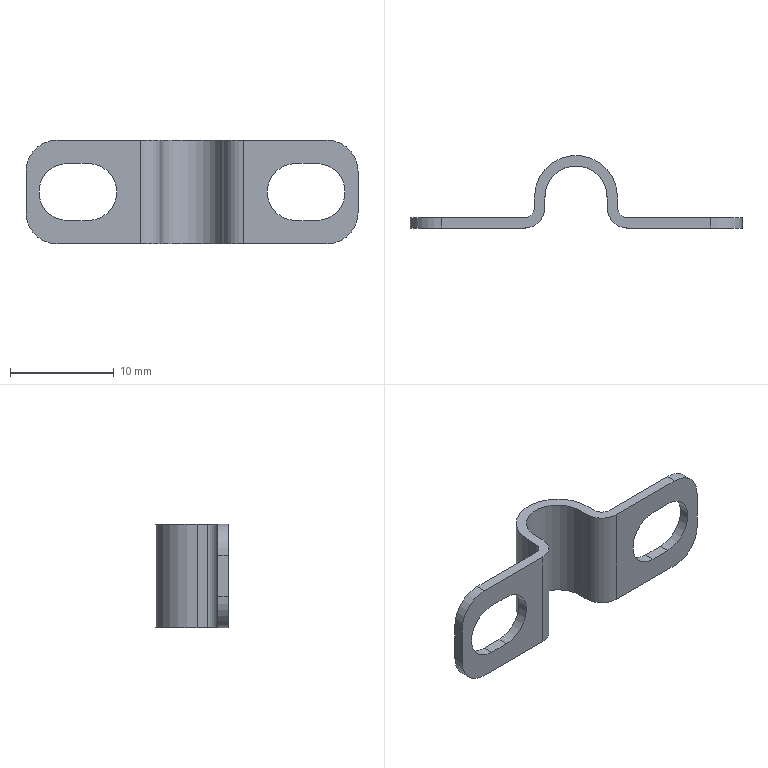Part | NX | features BREP 1 | 1 solid | 30 faces | box 32 x 7 x 10 mm | volume 319.837 mm3 | plane 16 | cylinder 14 | commonest cylinder face diameters 6 x5 5.5 x4 2 x2 4 x2 8 x1
STEP:
#1=CARTESIAN_POINT('',(-12.,0.,-2.75));
#2=VERTEX_POINT('',#1);
#3=CARTESIAN_POINT('',(-12.,0.,2.75));
#4=VERTEX_POINT('',#3);
#5=CARTESIAN_POINT('',(-12.,0.,0.));
#6=DIRECTION('',(0.,1.,0.));
#7=DIRECTION('',(0.,0.,1.));
#8=AXIS2_PLACEMENT_3D('',#5,#6,#7);
#9=CIRCLE('',#8,2.75);
#10=EDGE_CURVE('',#2,#4,#9,.T.);
#11=ORIENTED_EDGE('',*,*,#10,.F.);
#12=CARTESIAN_POINT('',(-12.,1.,-2.75));
#13=VERTEX_POINT('',#12);
#14=CARTESIAN_POINT('',(-12.,-9.,-2.75));
#15=DIRECTION('',(0.,1.,0.));
#16=VECTOR('',#15,1000.);
#17=LINE('',#14,#16);
#18=EDGE_CURVE('',#2,#13,#17,.T.);
#19=ORIENTED_EDGE('',*,*,#18,.T.);
#20=CARTESIAN_POINT('',(-12.,1.,2.75));
#21=VERTEX_POINT('',#20);
#22=CARTESIAN_POINT('',(-12.,1.,0.));
#23=DIRECTION('',(0.,1.,0.));
#24=DIRECTION('',(1.,0.,0.));
#25=AXIS2_PLACEMENT_3D('',#22,#23,#24);
#26=CIRCLE('',#25,2.75);
#27=EDGE_CURVE('',#13,#21,#26,.T.);
#28=ORIENTED_EDGE('',*,*,#27,.T.);
#29=CARTESIAN_POINT('',(-12.,-9.,2.75));
#30=DIRECTION('',(0.,1.,0.));
#31=VECTOR('',#30,1000.);
#32=LINE('',#29,#31);
#33=EDGE_CURVE('',#4,#21,#32,.T.);
#34=ORIENTED_EDGE('',*,*,#33,.F.);
#35=EDGE_LOOP('',(#11,#19,#28,#34));
#36=FACE_BOUND('',#35,.T.);
#37=CARTESIAN_POINT('',(-12.,-9.,0.));
#38=DIRECTION('',(0.,1.,0.));
#39=DIRECTION('',(-1.,0.,0.));
#40=AXIS2_PLACEMENT_3D('',#37,#38,#39);
#41=CYLINDRICAL_SURFACE('',#40,2.75);
#42=ADVANCED_FACE('',(#36),#41,.F.);
#43=CARTESIAN_POINT('',(10.,0.,-2.75));
#44=VERTEX_POINT('',#43);
#45=CARTESIAN_POINT('',(10.,0.,2.75));
#46=VERTEX_POINT('',#45);
#47=CARTESIAN_POINT('',(10.,0.,0.));
#48=DIRECTION('',(0.,1.,0.));
#49=DIRECTION('',(-1.,0.,0.));
#50=AXIS2_PLACEMENT_3D('',#47,#48,#49);
#51=CIRCLE('',#50,2.75);
#52=EDGE_CURVE('',#44,#46,#51,.T.);
#53=ORIENTED_EDGE('',*,*,#52,.F.);
#54=CARTESIAN_POINT('',(10.,1.,-2.75));
#55=VERTEX_POINT('',#54);
#56=CARTESIAN_POINT('',(10.,-9.,-2.75));
#57=DIRECTION('',(0.,1.,0.));
#58=VECTOR('',#57,1000.);
#59=LINE('',#56,#58);
#60=EDGE_CURVE('',#44,#55,#59,.T.);
#61=ORIENTED_EDGE('',*,*,#60,.T.);
#62=CARTESIAN_POINT('',(10.,1.,2.75));
#63=VERTEX_POINT('',#62);
#64=CARTESIAN_POINT('',(10.,1.,0.));
#65=DIRECTION('',(0.,1.,0.));
#66=DIRECTION('',(-1.,0.,0.));
#67=AXIS2_PLACEMENT_3D('',#64,#65,#66);
#68=CIRCLE('',#67,2.75);
#69=EDGE_CURVE('',#55,#63,#68,.T.);
#70=ORIENTED_EDGE('',*,*,#69,.T.);
#71=CARTESIAN_POINT('',(10.,-9.,2.75));
#72=DIRECTION('',(0.,1.,0.));
#73=VECTOR('',#72,1000.);
#74=LINE('',#71,#73);
#75=EDGE_CURVE('',#46,#63,#74,.T.);
#76=ORIENTED_EDGE('',*,*,#75,.F.);
#77=EDGE_LOOP('',(#53,#61,#70,#76));
#78=FACE_BOUND('',#77,.T.);
#79=CARTESIAN_POINT('',(10.,-9.,0.));
#80=DIRECTION('',(0.,1.,0.));
#81=DIRECTION('',(-1.,0.,0.));
#82=AXIS2_PLACEMENT_3D('',#79,#80,#81);
#83=CYLINDRICAL_SURFACE('',#82,2.75);
#84=ADVANCED_FACE('',(#78),#83,.F.);
#85=CARTESIAN_POINT('',(-16.,0.,2.));
#86=VERTEX_POINT('',#85);
#87=CARTESIAN_POINT('',(-16.,0.,-2.));
#88=VERTEX_POINT('',#87);
#89=CARTESIAN_POINT('',(-16.,0.,5.));
#90=DIRECTION('',(0.,0.,-1.));
#91=VECTOR('',#90,1000.);
#92=LINE('',#89,#91);
#93=EDGE_CURVE('',#86,#88,#92,.T.);
#94=ORIENTED_EDGE('',*,*,#93,.F.);
#95=CARTESIAN_POINT('',(-16.,1.,2.));
#96=VERTEX_POINT('',#95);
#97=CARTESIAN_POINT('',(-16.,1.,2.));
#98=DIRECTION('',(0.,1.,0.));
#99=VECTOR('',#98,1000.);
#100=LINE('',#97,#99);
#101=EDGE_CURVE('',#86,#96,#100,.T.);
#102=ORIENTED_EDGE('',*,*,#101,.T.);
#103=CARTESIAN_POINT('',(-16.,1.,-2.));
#104=VERTEX_POINT('',#103);
#105=CARTESIAN_POINT('',(-16.,1.,5.));
#106=DIRECTION('',(0.,0.,-1.));
#107=VECTOR('',#106,1000.);
#108=LINE('',#105,#107);
#109=EDGE_CURVE('',#96,#104,#108,.T.);
#110=ORIENTED_EDGE('',*,*,#109,.T.);
#111=CARTESIAN_POINT('',(-16.,1.,-2.));
#112=DIRECTION('',(0.,-1.,0.));
#113=VECTOR('',#112,1000.);
#114=LINE('',#111,#113);
#115=EDGE_CURVE('',#104,#88,#114,.T.);
#116=ORIENTED_EDGE('',*,*,#115,.T.);
#117=EDGE_LOOP('',(#94,#102,#110,#116));
#118=FACE_BOUND('',#117,.T.);
#119=CARTESIAN_POINT('',(-16.,1.,5.));
#120=DIRECTION('',(1.,0.,0.));
#121=DIRECTION('',(0.,0.,-1.));
#122=AXIS2_PLACEMENT_3D('',#119,#120,#121);
#123=PLANE('',#122);
#124=ADVANCED_FACE('',(#118),#123,.F.);
#125=CARTESIAN_POINT('',(-10.,0.,2.75));
#126=VERTEX_POINT('',#125);
#127=CARTESIAN_POINT('',(-16.,0.,2.75));
#128=DIRECTION('',(1.,0.,0.));
#129=VECTOR('',#128,1000.);
#130=LINE('',#127,#129);
#131=EDGE_CURVE('',#4,#126,#130,.T.);
#132=ORIENTED_EDGE('',*,*,#131,.T.);
#133=CARTESIAN_POINT('',(-10.,0.,-2.75));
#134=VERTEX_POINT('',#133);
#135=CARTESIAN_POINT('',(-10.,0.,0.));
#136=DIRECTION('',(0.,1.,0.));
#137=DIRECTION('',(0.,0.,1.));
#138=AXIS2_PLACEMENT_3D('',#135,#136,#137);
#139=CIRCLE('',#138,2.75);
#140=EDGE_CURVE('',#126,#134,#139,.T.);
#141=ORIENTED_EDGE('',*,*,#140,.T.);
#142=CARTESIAN_POINT('',(-16.,0.,-2.75));
#143=DIRECTION('',(-1.,0.,0.));
#144=VECTOR('',#143,1000.);
#145=LINE('',#142,#144);
#146=EDGE_CURVE('',#134,#2,#145,.T.);
#147=ORIENTED_EDGE('',*,*,#146,.T.);
#148=ORIENTED_EDGE('',*,*,#10,.T.);
#149=EDGE_LOOP('',(#132,#141,#147,#148));
#150=FACE_BOUND('',#149,.T.);
#151=CARTESIAN_POINT('',(-13.,0.,-5.));
#152=VERTEX_POINT('',#151);
#153=CARTESIAN_POINT('',(-5.,0.,-5.));
#154=VERTEX_POINT('',#153);
#155=CARTESIAN_POINT('',(-16.,0.,-5.));
#156=DIRECTION('',(1.,0.,0.));
#157=VECTOR('',#156,1000.);
#158=LINE('',#155,#157);
#159=EDGE_CURVE('',#152,#154,#158,.T.);
#160=ORIENTED_EDGE('',*,*,#159,.T.);
#161=CARTESIAN_POINT('',(-5.,0.,5.));
#162=VERTEX_POINT('',#161);
#163=CARTESIAN_POINT('',(-5.,0.,5.));
#164=DIRECTION('',(0.,0.,1.));
#165=VECTOR('',#164,1000.);
#166=LINE('',#163,#165);
#167=EDGE_CURVE('',#154,#162,#166,.T.);
#168=ORIENTED_EDGE('',*,*,#167,.T.);
#169=CARTESIAN_POINT('',(-13.,0.,5.));
#170=VERTEX_POINT('',#169);
#171=CARTESIAN_POINT('',(-16.,0.,5.));
#172=DIRECTION('',(1.,0.,0.));
#173=VECTOR('',#172,1000.);
#174=LINE('',#171,#173);
#175=EDGE_CURVE('',#170,#162,#174,.T.);
#176=ORIENTED_EDGE('',*,*,#175,.F.);
#177=CARTESIAN_POINT('',(-13.,0.,2.));
#178=DIRECTION('',(0.,-1.,0.));
#179=DIRECTION('',(0.,0.,1.));
#180=AXIS2_PLACEMENT_3D('',#177,#178,#179);
#181=CIRCLE('',#180,3.);
#182=EDGE_CURVE('',#170,#86,#181,.T.);
#183=ORIENTED_EDGE('',*,*,#182,.T.);
#184=ORIENTED_EDGE('',*,*,#93,.T.);
#185=CARTESIAN_POINT('',(-13.,0.,-2.));
#186=DIRECTION('',(0.,-1.,0.));
#187=DIRECTION('',(0.,0.,1.));
#188=AXIS2_PLACEMENT_3D('',#185,#186,#187);
#189=CIRCLE('',#188,3.);
#190=EDGE_CURVE('',#88,#152,#189,.T.);
#191=ORIENTED_EDGE('',*,*,#190,.T.);
#192=EDGE_LOOP('',(#160,#168,#176,#183,#184,#191));
#193=FACE_BOUND('',#192,.T.);
#194=CARTESIAN_POINT('',(-16.,0.,5.));
#195=DIRECTION('',(0.,1.,0.));
#196=DIRECTION('',(0.,0.,1.));
#197=AXIS2_PLACEMENT_3D('',#194,#195,#196);
#198=PLANE('',#197);
#199=ADVANCED_FACE('',(#150,#193),#198,.F.);
#200=CARTESIAN_POINT('',(-3.,2.,5.));
#201=VERTEX_POINT('',#200);
#202=CARTESIAN_POINT('',(-3.,3.,5.));
#203=VERTEX_POINT('',#202);
#204=CARTESIAN_POINT('',(-3.,0.,5.));
#205=DIRECTION('',(0.,1.,0.));
#206=VECTOR('',#205,1000.);
#207=LINE('',#204,#206);
#208=EDGE_CURVE('',#201,#203,#207,.T.);
#209=ORIENTED_EDGE('',*,*,#208,.F.);
#210=CARTESIAN_POINT('',(-3.,2.,-5.));
#211=VERTEX_POINT('',#210);
#212=CARTESIAN_POINT('',(-3.,2.,5.));
#213=DIRECTION('',(0.,0.,-1.));
#214=VECTOR('',#213,1000.);
#215=LINE('',#212,#214);
#216=EDGE_CURVE('',#201,#211,#215,.T.);
#217=ORIENTED_EDGE('',*,*,#216,.T.);
#218=CARTESIAN_POINT('',(-3.,3.,-5.));
#219=VERTEX_POINT('',#218);
#220=CARTESIAN_POINT('',(-3.,0.,-5.));
#221=DIRECTION('',(0.,1.,0.));
#222=VECTOR('',#221,1000.);
#223=LINE('',#220,#222);
#224=EDGE_CURVE('',#211,#219,#223,.T.);
#225=ORIENTED_EDGE('',*,*,#224,.T.);
#226=CARTESIAN_POINT('',(-3.,3.,5.));
#227=DIRECTION('',(0.,0.,-1.));
#228=VECTOR('',#227,1000.);
#229=LINE('',#226,#228);
#230=EDGE_CURVE('',#203,#219,#229,.T.);
#231=ORIENTED_EDGE('',*,*,#230,.F.);
#232=EDGE_LOOP('',(#209,#217,#225,#231));
#233=FACE_BOUND('',#232,.T.);
#234=CARTESIAN_POINT('',(-3.,0.,5.));
#235=DIRECTION('',(-1.,0.,0.));
#236=DIRECTION('',(0.,0.,1.));
#237=AXIS2_PLACEMENT_3D('',#234,#235,#236);
#238=PLANE('',#237);
#239=ADVANCED_FACE('',(#233),#238,.F.);
#240=CARTESIAN_POINT('',(3.,3.,-5.));
#241=VERTEX_POINT('',#240);
#242=CARTESIAN_POINT('',(0.,3.,-5.));
#243=DIRECTION('',(0.,0.,-1.));
#244=DIRECTION('',(1.,0.,0.));
#245=AXIS2_PLACEMENT_3D('',#242,#243,#244);
#246=CIRCLE('',#245,3.);
#247=EDGE_CURVE('',#219,#241,#246,.T.);
#248=ORIENTED_EDGE('',*,*,#247,.T.);
#249=CARTESIAN_POINT('',(3.,3.,5.));
#250=VERTEX_POINT('',#249);
#251=CARTESIAN_POINT('',(3.,3.,5.));
#252=DIRECTION('',(0.,0.,-1.));
#253=VECTOR('',#252,1000.);
#254=LINE('',#251,#253);
#255=EDGE_CURVE('',#250,#241,#254,.T.);
#256=ORIENTED_EDGE('',*,*,#255,.F.);
#257=CARTESIAN_POINT('',(0.,3.,5.));
#258=DIRECTION('',(0.,0.,-1.));
#259=DIRECTION('',(1.,0.,0.));
#260=AXIS2_PLACEMENT_3D('',#257,#258,#259);
#261=CIRCLE('',#260,3.);
#262=EDGE_CURVE('',#203,#250,#261,.T.);
#263=ORIENTED_EDGE('',*,*,#262,.F.);
#264=ORIENTED_EDGE('',*,*,#230,.T.);
#265=EDGE_LOOP('',(#248,#256,#263,#264));
#266=FACE_BOUND('',#265,.T.);
#267=CARTESIAN_POINT('',(0.,3.,5.));
#268=DIRECTION('',(0.,0.,-1.));
#269=DIRECTION('',(-1.,0.,0.));
#270=AXIS2_PLACEMENT_3D('',#267,#268,#269);
#271=CYLINDRICAL_SURFACE('',#270,3.);
#272=ADVANCED_FACE('',(#266),#271,.F.);
#273=CARTESIAN_POINT('',(3.,2.,-5.));
#274=VERTEX_POINT('',#273);
#275=CARTESIAN_POINT('',(3.,0.,-5.));
#276=DIRECTION('',(0.,-1.,0.));
#277=VECTOR('',#276,1000.);
#278=LINE('',#275,#277);
#279=EDGE_CURVE('',#241,#274,#278,.T.);
#280=ORIENTED_EDGE('',*,*,#279,.T.);
#281=CARTESIAN_POINT('',(3.,2.,5.));
#282=VERTEX_POINT('',#281);
#283=CARTESIAN_POINT('',(3.,2.,5.));
#284=DIRECTION('',(0.,0.,1.));
#285=VECTOR('',#284,1000.);
#286=LINE('',#283,#285);
#287=EDGE_CURVE('',#274,#282,#286,.T.);
#288=ORIENTED_EDGE('',*,*,#287,.T.);
#289=CARTESIAN_POINT('',(3.,0.,5.));
#290=DIRECTION('',(0.,-1.,0.));
#291=VECTOR('',#290,1000.);
#292=LINE('',#289,#291);
#293=EDGE_CURVE('',#250,#282,#292,.T.);
#294=ORIENTED_EDGE('',*,*,#293,.F.);
#295=ORIENTED_EDGE('',*,*,#255,.T.);
#296=EDGE_LOOP('',(#280,#288,#294,#295));
#297=FACE_BOUND('',#296,.T.);
#298=CARTESIAN_POINT('',(3.,0.,5.));
#299=DIRECTION('',(1.,0.,0.));
#300=DIRECTION('',(0.,1.,0.));
#301=AXIS2_PLACEMENT_3D('',#298,#299,#300);
#302=PLANE('',#301);
#303=ADVANCED_FACE('',(#297),#302,.F.);
#304=CARTESIAN_POINT('',(12.,0.,-2.75));
#305=VERTEX_POINT('',#304);
#306=CARTESIAN_POINT('',(3.,0.,-2.75));
#307=DIRECTION('',(-1.,0.,0.));
#308=VECTOR('',#307,1000.);
#309=LINE('',#306,#308);
#310=EDGE_CURVE('',#305,#44,#309,.T.);
#311=ORIENTED_EDGE('',*,*,#310,.T.);
#312=ORIENTED_EDGE('',*,*,#52,.T.);
#313=CARTESIAN_POINT('',(12.,0.,2.75));
#314=VERTEX_POINT('',#313);
#315=CARTESIAN_POINT('',(3.,0.,2.75));
#316=DIRECTION('',(1.,0.,0.));
#317=VECTOR('',#316,1000.);
#318=LINE('',#315,#317);
#319=EDGE_CURVE('',#46,#314,#318,.T.);
#320=ORIENTED_EDGE('',*,*,#319,.T.);
#321=CARTESIAN_POINT('',(12.,0.,0.));
#322=DIRECTION('',(0.,1.,0.));
#323=DIRECTION('',(-1.,0.,0.));
#324=AXIS2_PLACEMENT_3D('',#321,#322,#323);
#325=CIRCLE('',#324,2.75);
#326=EDGE_CURVE('',#314,#305,#325,.T.);
#327=ORIENTED_EDGE('',*,*,#326,.T.);
#328=EDGE_LOOP('',(#311,#312,#320,#327));
#329=FACE_BOUND('',#328,.T.);
#330=CARTESIAN_POINT('',(5.,0.,5.));
#331=VERTEX_POINT('',#330);
#332=CARTESIAN_POINT('',(13.,0.,5.));
#333=VERTEX_POINT('',#332);
#334=CARTESIAN_POINT('',(3.,0.,5.));
#335=DIRECTION('',(1.,0.,0.));
#336=VECTOR('',#335,1000.);
#337=LINE('',#334,#336);
#338=EDGE_CURVE('',#331,#333,#337,.T.);
#339=ORIENTED_EDGE('',*,*,#338,.F.);
#340=CARTESIAN_POINT('',(5.,0.,-5.));
#341=VERTEX_POINT('',#340);
#342=CARTESIAN_POINT('',(5.,0.,5.));
#343=DIRECTION('',(0.,0.,-1.));
#344=VECTOR('',#343,1000.);
#345=LINE('',#342,#344);
#346=EDGE_CURVE('',#331,#341,#345,.T.);
#347=ORIENTED_EDGE('',*,*,#346,.T.);
#348=CARTESIAN_POINT('',(13.,0.,-5.));
#349=VERTEX_POINT('',#348);
#350=CARTESIAN_POINT('',(3.,0.,-5.));
#351=DIRECTION('',(1.,0.,0.));
#352=VECTOR('',#351,1000.);
#353=LINE('',#350,#352);
#354=EDGE_CURVE('',#341,#349,#353,.T.);
#355=ORIENTED_EDGE('',*,*,#354,.T.);
#356=CARTESIAN_POINT('',(16.,0.,-2.));
#357=VERTEX_POINT('',#356);
#358=CARTESIAN_POINT('',(13.,0.,-2.));
#359=DIRECTION('',(0.,-1.,0.));
#360=DIRECTION('',(-1.,0.,0.));
#361=AXIS2_PLACEMENT_3D('',#358,#359,#360);
#362=CIRCLE('',#361,3.);
#363=EDGE_CURVE('',#349,#357,#362,.T.);
#364=ORIENTED_EDGE('',*,*,#363,.T.);
#365=CARTESIAN_POINT('',(16.,0.,2.));
#366=VERTEX_POINT('',#365);
#367=CARTESIAN_POINT('',(16.,0.,5.));
#368=DIRECTION('',(0.,0.,-1.));
#369=VECTOR('',#368,1000.);
#370=LINE('',#367,#369);
#371=EDGE_CURVE('',#366,#357,#370,.T.);
#372=ORIENTED_EDGE('',*,*,#371,.F.);
#373=CARTESIAN_POINT('',(13.,0.,2.));
#374=DIRECTION('',(0.,-1.,0.));
#375=DIRECTION('',(-1.,0.,0.));
#376=AXIS2_PLACEMENT_3D('',#373,#374,#375);
#377=CIRCLE('',#376,3.);
#378=EDGE_CURVE('',#366,#333,#377,.T.);
#379=ORIENTED_EDGE('',*,*,#378,.T.);
#380=EDGE_LOOP('',(#339,#347,#355,#364,#372,#379));
#381=FACE_BOUND('',#380,.T.);
#382=CARTESIAN_POINT('',(3.,0.,5.));
#383=DIRECTION('',(0.,1.,0.));
#384=DIRECTION('',(-1.,0.,0.));
#385=AXIS2_PLACEMENT_3D('',#382,#383,#384);
#386=PLANE('',#385);
#387=ADVANCED_FACE('',(#329,#381),#386,.F.);
#388=ORIENTED_EDGE('',*,*,#371,.T.);
#389=CARTESIAN_POINT('',(16.,1.,-2.));
#390=VERTEX_POINT('',#389);
#391=CARTESIAN_POINT('',(16.,0.,-2.));
#392=DIRECTION('',(0.,1.,0.));
#393=VECTOR('',#392,1000.);
#394=LINE('',#391,#393);
#395=EDGE_CURVE('',#357,#390,#394,.T.);
#396=ORIENTED_EDGE('',*,*,#395,.T.);
#397=CARTESIAN_POINT('',(16.,1.,2.));
#398=VERTEX_POINT('',#397);
#399=CARTESIAN_POINT('',(16.,1.,5.));
#400=DIRECTION('',(0.,0.,-1.));
#401=VECTOR('',#400,1000.);
#402=LINE('',#399,#401);
#403=EDGE_CURVE('',#398,#390,#402,.T.);
#404=ORIENTED_EDGE('',*,*,#403,.F.);
#405=CARTESIAN_POINT('',(16.,0.,2.));
#406=DIRECTION('',(0.,-1.,0.));
#407=VECTOR('',#406,1000.);
#408=LINE('',#405,#407);
#409=EDGE_CURVE('',#398,#366,#408,.T.);
#410=ORIENTED_EDGE('',*,*,#409,.T.);
#411=EDGE_LOOP('',(#388,#396,#404,#410));
#412=FACE_BOUND('',#411,.T.);
#413=CARTESIAN_POINT('',(16.,0.,5.));
#414=DIRECTION('',(-1.,0.,0.));
#415=DIRECTION('',(0.,0.,1.));
#416=AXIS2_PLACEMENT_3D('',#413,#414,#415);
#417=PLANE('',#416);
#418=ADVANCED_FACE('',(#412),#417,.F.);
#419=CARTESIAN_POINT('',(12.,1.,2.75));
#420=VERTEX_POINT('',#419);
#421=CARTESIAN_POINT('',(10.,1.,2.75));
#422=DIRECTION('',(1.,0.,0.));
#423=VECTOR('',#422,1000.);
#424=LINE('',#421,#423);
#425=EDGE_CURVE('',#63,#420,#424,.T.);
#426=ORIENTED_EDGE('',*,*,#425,.F.);
#427=ORIENTED_EDGE('',*,*,#69,.F.);
#428=CARTESIAN_POINT('',(12.,1.,-2.75));
#429=VERTEX_POINT('',#428);
#430=CARTESIAN_POINT('',(10.,1.,-2.75));
#431=DIRECTION('',(-1.,0.,0.));
#432=VECTOR('',#431,1000.);
#433=LINE('',#430,#432);
#434=EDGE_CURVE('',#429,#55,#433,.T.);
#435=ORIENTED_EDGE('',*,*,#434,.F.);
#436=CARTESIAN_POINT('',(12.,1.,0.));
#437=DIRECTION('',(0.,1.,0.));
#438=DIRECTION('',(-1.,0.,0.));
#439=AXIS2_PLACEMENT_3D('',#436,#437,#438);
#440=CIRCLE('',#439,2.75);
#441=EDGE_CURVE('',#420,#429,#440,.T.);
#442=ORIENTED_EDGE('',*,*,#441,.F.);
#443=EDGE_LOOP('',(#426,#427,#435,#442));
#444=FACE_BOUND('',#443,.T.);
#445=CARTESIAN_POINT('',(13.,1.,-5.));
#446=VERTEX_POINT('',#445);
#447=CARTESIAN_POINT('',(5.,1.,-5.));
#448=VERTEX_POINT('',#447);
#449=CARTESIAN_POINT('',(4.,1.,-5.));
#450=DIRECTION('',(-1.,0.,0.));
#451=VECTOR('',#450,1000.);
#452=LINE('',#449,#451);
#453=EDGE_CURVE('',#446,#448,#452,.T.);
#454=ORIENTED_EDGE('',*,*,#453,.T.);
#455=CARTESIAN_POINT('',(5.,1.,5.));
#456=VERTEX_POINT('',#455);
#457=CARTESIAN_POINT('',(5.,1.,5.));
#458=DIRECTION('',(0.,0.,1.));
#459=VECTOR('',#458,1000.);
#460=LINE('',#457,#459);
#461=EDGE_CURVE('',#448,#456,#460,.T.);
#462=ORIENTED_EDGE('',*,*,#461,.T.);
#463=CARTESIAN_POINT('',(13.,1.,5.));
#464=VERTEX_POINT('',#463);
#465=CARTESIAN_POINT('',(4.,1.,5.));
#466=DIRECTION('',(-1.,0.,0.));
#467=VECTOR('',#466,1000.);
#468=LINE('',#465,#467);
#469=EDGE_CURVE('',#464,#456,#468,.T.);
#470=ORIENTED_EDGE('',*,*,#469,.F.);
#471=CARTESIAN_POINT('',(13.,1.,2.));
#472=DIRECTION('',(0.,1.,0.));
#473=DIRECTION('',(1.,0.,0.));
#474=AXIS2_PLACEMENT_3D('',#471,#472,#473);
#475=CIRCLE('',#474,3.);
#476=EDGE_CURVE('',#464,#398,#475,.T.);
#477=ORIENTED_EDGE('',*,*,#476,.T.);
#478=ORIENTED_EDGE('',*,*,#403,.T.);
#479=CARTESIAN_POINT('',(13.,1.,-2.));
#480=DIRECTION('',(0.,1.,0.));
#481=DIRECTION('',(1.,0.,0.));
#482=AXIS2_PLACEMENT_3D('',#479,#480,#481);
#483=CIRCLE('',#482,3.);
#484=EDGE_CURVE('',#390,#446,#483,.T.);
#485=ORIENTED_EDGE('',*,*,#484,.T.);
#486=EDGE_LOOP('',(#454,#462,#470,#477,#478,#485));
#487=FACE_BOUND('',#486,.T.);
#488=CARTESIAN_POINT('',(4.,1.,5.));
#489=DIRECTION('',(0.,-1.,0.));
#490=DIRECTION('',(1.,0.,0.));
#491=AXIS2_PLACEMENT_3D('',#488,#489,#490);
#492=PLANE('',#491);
#493=ADVANCED_FACE('',(#444,#487),#492,.F.);
#494=CARTESIAN_POINT('',(4.,2.,5.));
#495=VERTEX_POINT('',#494);
#496=CARTESIAN_POINT('',(4.,3.,5.));
#497=VERTEX_POINT('',#496);
#498=CARTESIAN_POINT('',(4.,1.,5.));
#499=DIRECTION('',(0.,1.,0.));
#500=VECTOR('',#499,1000.);
#501=LINE('',#498,#500);
#502=EDGE_CURVE('',#495,#497,#501,.T.);
#503=ORIENTED_EDGE('',*,*,#502,.F.);
#504=CARTESIAN_POINT('',(4.,2.,-5.));
#505=VERTEX_POINT('',#504);
#506=CARTESIAN_POINT('',(4.,2.,-5.));
#507=DIRECTION('',(0.,0.,-1.));
#508=VECTOR('',#507,1000.);
#509=LINE('',#506,#508);
#510=EDGE_CURVE('',#495,#505,#509,.T.);
#511=ORIENTED_EDGE('',*,*,#510,.T.);
#512=CARTESIAN_POINT('',(4.,3.,-5.));
#513=VERTEX_POINT('',#512);
#514=CARTESIAN_POINT('',(4.,1.,-5.));
#515=DIRECTION('',(0.,1.,0.));
#516=VECTOR('',#515,1000.);
#517=LINE('',#514,#516);
#518=EDGE_CURVE('',#505,#513,#517,.T.);
#519=ORIENTED_EDGE('',*,*,#518,.T.);
#520=CARTESIAN_POINT('',(4.,3.,5.));
#521=DIRECTION('',(0.,0.,-1.));
#522=VECTOR('',#521,1000.);
#523=LINE('',#520,#522);
#524=EDGE_CURVE('',#497,#513,#523,.T.);
#525=ORIENTED_EDGE('',*,*,#524,.F.);
#526=EDGE_LOOP('',(#503,#511,#519,#525));
#527=FACE_BOUND('',#526,.T.);
#528=CARTESIAN_POINT('',(4.,1.,5.));
#529=DIRECTION('',(-1.,0.,0.));
#530=DIRECTION('',(0.,0.,1.));
#531=AXIS2_PLACEMENT_3D('',#528,#529,#530);
#532=PLANE('',#531);
#533=ADVANCED_FACE('',(#527),#532,.F.);
#534=CARTESIAN_POINT('',(-4.,3.,-5.));
#535=VERTEX_POINT('',#534);
#536=CARTESIAN_POINT('',(0.,3.,-5.));
#537=DIRECTION('',(0.,0.,1.));
#538=DIRECTION('',(1.,0.,0.));
#539=AXIS2_PLACEMENT_3D('',#536,#537,#538);
#540=CIRCLE('',#539,4.);
#541=EDGE_CURVE('',#513,#535,#540,.T.);
#542=ORIENTED_EDGE('',*,*,#541,.T.);
#543=CARTESIAN_POINT('',(-4.,3.,5.));
#544=VERTEX_POINT('',#543);
#545=CARTESIAN_POINT('',(-4.,3.,5.));
#546=DIRECTION('',(0.,0.,-1.));
#547=VECTOR('',#546,1000.);
#548=LINE('',#545,#547);
#549=EDGE_CURVE('',#544,#535,#548,.T.);
#550=ORIENTED_EDGE('',*,*,#549,.F.);
#551=CARTESIAN_POINT('',(0.,3.,5.));
#552=DIRECTION('',(0.,0.,1.));
#553=DIRECTION('',(1.,0.,0.));
#554=AXIS2_PLACEMENT_3D('',#551,#552,#553);
#555=CIRCLE('',#554,4.);
#556=EDGE_CURVE('',#497,#544,#555,.T.);
#557=ORIENTED_EDGE('',*,*,#556,.F.);
#558=ORIENTED_EDGE('',*,*,#524,.T.);
#559=EDGE_LOOP('',(#542,#550,#557,#558));
#560=FACE_BOUND('',#559,.T.);
#561=CARTESIAN_POINT('',(0.,3.,5.));
#562=DIRECTION('',(0.,0.,-1.));
#563=DIRECTION('',(-1.,0.,0.));
#564=AXIS2_PLACEMENT_3D('',#561,#562,#563);
#565=CYLINDRICAL_SURFACE('',#564,4.);
#566=ADVANCED_FACE('',(#560),#565,.T.);
#567=CARTESIAN_POINT('',(-4.,2.,-5.));
#568=VERTEX_POINT('',#567);
#569=CARTESIAN_POINT('',(-4.,1.,-5.));
#570=DIRECTION('',(0.,-1.,0.));
#571=VECTOR('',#570,1000.);
#572=LINE('',#569,#571);
#573=EDGE_CURVE('',#535,#568,#572,.T.);
#574=ORIENTED_EDGE('',*,*,#573,.T.);
#575=CARTESIAN_POINT('',(-4.,2.,5.));
#576=VERTEX_POINT('',#575);
#577=CARTESIAN_POINT('',(-4.,2.,5.));
#578=DIRECTION('',(0.,0.,1.));
#579=VECTOR('',#578,1000.);
#580=LINE('',#577,#579);
#581=EDGE_CURVE('',#568,#576,#580,.T.);
#582=ORIENTED_EDGE('',*,*,#581,.T.);
#583=CARTESIAN_POINT('',(-4.,1.,5.));
#584=DIRECTION('',(0.,-1.,0.));
#585=VECTOR('',#584,1000.);
#586=LINE('',#583,#585);
#587=EDGE_CURVE('',#544,#576,#586,.T.);
#588=ORIENTED_EDGE('',*,*,#587,.F.);
#589=ORIENTED_EDGE('',*,*,#549,.T.);
#590=EDGE_LOOP('',(#574,#582,#588,#589));
#591=FACE_BOUND('',#590,.T.);
#592=CARTESIAN_POINT('',(-4.,1.,5.));
#593=DIRECTION('',(1.,0.,0.));
#594=DIRECTION('',(0.,1.,0.));
#595=AXIS2_PLACEMENT_3D('',#592,#593,#594);
#596=PLANE('',#595);
#597=ADVANCED_FACE('',(#591),#596,.F.);
#598=CARTESIAN_POINT('',(-10.,1.,-2.75));
#599=VERTEX_POINT('',#598);
#600=CARTESIAN_POINT('',(-10.,1.,-2.75));
#601=DIRECTION('',(-1.,0.,0.));
#602=VECTOR('',#601,1000.);
#603=LINE('',#600,#602);
#604=EDGE_CURVE('',#599,#13,#603,.T.);
#605=ORIENTED_EDGE('',*,*,#604,.F.);
#606=CARTESIAN_POINT('',(-10.,1.,2.75));
#607=VERTEX_POINT('',#606);
#608=CARTESIAN_POINT('',(-10.,1.,0.));
#609=DIRECTION('',(0.,1.,0.));
#610=DIRECTION('',(1.,0.,0.));
#611=AXIS2_PLACEMENT_3D('',#608,#609,#610);
#612=CIRCLE('',#611,2.75);
#613=EDGE_CURVE('',#607,#599,#612,.T.);
#614=ORIENTED_EDGE('',*,*,#613,.F.);
#615=CARTESIAN_POINT('',(-10.,1.,2.75));
#616=DIRECTION('',(1.,0.,0.));
#617=VECTOR('',#616,1000.);
#618=LINE('',#615,#617);
#619=EDGE_CURVE('',#21,#607,#618,.T.);
#620=ORIENTED_EDGE('',*,*,#619,.F.);
#621=ORIENTED_EDGE('',*,*,#27,.F.);
#622=EDGE_LOOP('',(#605,#614,#620,#621));
#623=FACE_BOUND('',#622,.T.);
#624=CARTESIAN_POINT('',(-5.,1.,5.));
#625=VERTEX_POINT('',#624);
#626=CARTESIAN_POINT('',(-13.,1.,5.));
#627=VERTEX_POINT('',#626);
#628=CARTESIAN_POINT('',(-16.,1.,5.));
#629=DIRECTION('',(-1.,0.,0.));
#630=VECTOR('',#629,1000.);
#631=LINE('',#628,#630);
#632=EDGE_CURVE('',#625,#627,#631,.T.);
#633=ORIENTED_EDGE('',*,*,#632,.F.);
#634=CARTESIAN_POINT('',(-5.,1.,-5.));
#635=VERTEX_POINT('',#634);
#636=CARTESIAN_POINT('',(-5.,1.,-5.));
#637=DIRECTION('',(0.,0.,-1.));
#638=VECTOR('',#637,1000.);
#639=LINE('',#636,#638);
#640=EDGE_CURVE('',#625,#635,#639,.T.);
#641=ORIENTED_EDGE('',*,*,#640,.T.);
#642=CARTESIAN_POINT('',(-13.,1.,-5.));
#643=VERTEX_POINT('',#642);
#644=CARTESIAN_POINT('',(-16.,1.,-5.));
#645=DIRECTION('',(-1.,0.,0.));
#646=VECTOR('',#645,1000.);
#647=LINE('',#644,#646);
#648=EDGE_CURVE('',#635,#643,#647,.T.);
#649=ORIENTED_EDGE('',*,*,#648,.T.);
#650=CARTESIAN_POINT('',(-13.,1.,-2.));
#651=DIRECTION('',(0.,1.,0.));
#652=DIRECTION('',(0.,0.,-1.));
#653=AXIS2_PLACEMENT_3D('',#650,#651,#652);
#654=CIRCLE('',#653,3.);
#655=EDGE_CURVE('',#643,#104,#654,.T.);
#656=ORIENTED_EDGE('',*,*,#655,.T.);
#657=ORIENTED_EDGE('',*,*,#109,.F.);
#658=CARTESIAN_POINT('',(-13.,1.,2.));
#659=DIRECTION('',(0.,1.,0.));
#660=DIRECTION('',(0.,0.,-1.));
#661=AXIS2_PLACEMENT_3D('',#658,#659,#660);
#662=CIRCLE('',#661,3.);
#663=EDGE_CURVE('',#96,#627,#662,.T.);
#664=ORIENTED_EDGE('',*,*,#663,.T.);
#665=EDGE_LOOP('',(#633,#641,#649,#656,#657,#664));
#666=FACE_BOUND('',#665,.T.);
#667=CARTESIAN_POINT('',(-16.,1.,5.));
#668=DIRECTION('',(0.,-1.,0.));
#669=DIRECTION('',(0.,0.,-1.));
#670=AXIS2_PLACEMENT_3D('',#667,#668,#669);
#671=PLANE('',#670);
#672=ADVANCED_FACE('',(#623,#666),#671,.F.);
#673=ORIENTED_EDGE('',*,*,#175,.T.);
#674=CARTESIAN_POINT('',(-5.,2.,5.));
#675=DIRECTION('',(0.,0.,1.));
#676=DIRECTION('',(1.,0.,0.));
#677=AXIS2_PLACEMENT_3D('',#674,#675,#676);
#678=CIRCLE('',#677,2.);
#679=EDGE_CURVE('',#162,#201,#678,.T.);
#680=ORIENTED_EDGE('',*,*,#679,.T.);
#681=ORIENTED_EDGE('',*,*,#208,.T.);
#682=ORIENTED_EDGE('',*,*,#262,.T.);
#683=ORIENTED_EDGE('',*,*,#293,.T.);
#684=CARTESIAN_POINT('',(5.,2.,5.));
#685=DIRECTION('',(0.,0.,1.));
#686=DIRECTION('',(1.,0.,0.));
#687=AXIS2_PLACEMENT_3D('',#684,#685,#686);
#688=CIRCLE('',#687,2.);
#689=EDGE_CURVE('',#282,#331,#688,.T.);
#690=ORIENTED_EDGE('',*,*,#689,.T.);
#691=ORIENTED_EDGE('',*,*,#338,.T.);
#692=CARTESIAN_POINT('',(13.,1.,5.));
#693=DIRECTION('',(0.,1.,0.));
#694=VECTOR('',#693,1000.);
#695=LINE('',#692,#694);
#696=EDGE_CURVE('',#333,#464,#695,.T.);
#697=ORIENTED_EDGE('',*,*,#696,.T.);
#698=ORIENTED_EDGE('',*,*,#469,.T.);
#699=CARTESIAN_POINT('',(5.,2.,5.));
#700=DIRECTION('',(0.,0.,-1.));
#701=DIRECTION('',(1.,0.,0.));
#702=AXIS2_PLACEMENT_3D('',#699,#700,#701);
#703=CIRCLE('',#702,1.);
#704=EDGE_CURVE('',#456,#495,#703,.T.);
#705=ORIENTED_EDGE('',*,*,#704,.T.);
#706=ORIENTED_EDGE('',*,*,#502,.T.);
#707=ORIENTED_EDGE('',*,*,#556,.T.);
#708=ORIENTED_EDGE('',*,*,#587,.T.);
#709=CARTESIAN_POINT('',(-5.,2.,5.));
#710=DIRECTION('',(0.,0.,-1.));
#711=DIRECTION('',(1.,0.,0.));
#712=AXIS2_PLACEMENT_3D('',#709,#710,#711);
#713=CIRCLE('',#712,1.);
#714=EDGE_CURVE('',#576,#625,#713,.T.);
#715=ORIENTED_EDGE('',*,*,#714,.T.);
#716=ORIENTED_EDGE('',*,*,#632,.T.);
#717=CARTESIAN_POINT('',(-13.,0.,5.));
#718=DIRECTION('',(0.,-1.,0.));
#719=VECTOR('',#718,1000.);
#720=LINE('',#717,#719);
#721=EDGE_CURVE('',#627,#170,#720,.T.);
#722=ORIENTED_EDGE('',*,*,#721,.T.);
#723=EDGE_LOOP('',(#673,#680,#681,#682,#683,#690,#691,#697,#698,#705,#706,#707,#708,#715,#716,#722));
#724=FACE_BOUND('',#723,.T.);
#725=CARTESIAN_POINT('',(0.,3.,5.));
#726=DIRECTION('',(0.,0.,1.));
#727=DIRECTION('',(1.,0.,0.));
#728=AXIS2_PLACEMENT_3D('',#725,#726,#727);
#729=PLANE('',#728);
#730=ADVANCED_FACE('',(#724),#729,.T.);
#731=ORIENTED_EDGE('',*,*,#224,.F.);
#732=CARTESIAN_POINT('',(-5.,2.,-5.));
#733=DIRECTION('',(0.,0.,-1.));
#734=DIRECTION('',(1.,0.,0.));
#735=AXIS2_PLACEMENT_3D('',#732,#733,#734);
#736=CIRCLE('',#735,2.);
#737=EDGE_CURVE('',#211,#154,#736,.T.);
#738=ORIENTED_EDGE('',*,*,#737,.T.);
#739=ORIENTED_EDGE('',*,*,#159,.F.);
#740=CARTESIAN_POINT('',(-13.,3.,-5.));
#741=DIRECTION('',(0.,1.,0.));
#742=VECTOR('',#741,1000.);
#743=LINE('',#740,#742);
#744=EDGE_CURVE('',#152,#643,#743,.T.);
#745=ORIENTED_EDGE('',*,*,#744,.T.);
#746=ORIENTED_EDGE('',*,*,#648,.F.);
#747=CARTESIAN_POINT('',(-5.,2.,-5.));
#748=DIRECTION('',(0.,0.,1.));
#749=DIRECTION('',(1.,0.,0.));
#750=AXIS2_PLACEMENT_3D('',#747,#748,#749);
#751=CIRCLE('',#750,1.);
#752=EDGE_CURVE('',#635,#568,#751,.T.);
#753=ORIENTED_EDGE('',*,*,#752,.T.);
#754=ORIENTED_EDGE('',*,*,#573,.F.);
#755=ORIENTED_EDGE('',*,*,#541,.F.);
#756=ORIENTED_EDGE('',*,*,#518,.F.);
#757=CARTESIAN_POINT('',(5.,2.,-5.));
#758=DIRECTION('',(0.,0.,1.));
#759=DIRECTION('',(1.,0.,0.));
#760=AXIS2_PLACEMENT_3D('',#757,#758,#759);
#761=CIRCLE('',#760,1.);
#762=EDGE_CURVE('',#505,#448,#761,.T.);
#763=ORIENTED_EDGE('',*,*,#762,.T.);
#764=ORIENTED_EDGE('',*,*,#453,.F.);
#765=CARTESIAN_POINT('',(13.,3.,-5.));
#766=DIRECTION('',(0.,-1.,0.));
#767=VECTOR('',#766,1000.);
#768=LINE('',#765,#767);
#769=EDGE_CURVE('',#446,#349,#768,.T.);
#770=ORIENTED_EDGE('',*,*,#769,.T.);
#771=ORIENTED_EDGE('',*,*,#354,.F.);
#772=CARTESIAN_POINT('',(5.,2.,-5.));
#773=DIRECTION('',(0.,0.,-1.));
#774=DIRECTION('',(1.,0.,0.));
#775=AXIS2_PLACEMENT_3D('',#772,#773,#774);
#776=CIRCLE('',#775,2.);
#777=EDGE_CURVE('',#341,#274,#776,.T.);
#778=ORIENTED_EDGE('',*,*,#777,.T.);
#779=ORIENTED_EDGE('',*,*,#279,.F.);
#780=ORIENTED_EDGE('',*,*,#247,.F.);
#781=EDGE_LOOP('',(#731,#738,#739,#745,#746,#753,#754,#755,#756,#763,#764,#770,#771,#778,#779,#780));
#782=FACE_BOUND('',#781,.T.);
#783=CARTESIAN_POINT('',(0.,3.,-5.));
#784=DIRECTION('',(0.,0.,1.));
#785=DIRECTION('',(1.,0.,0.));
#786=AXIS2_PLACEMENT_3D('',#783,#784,#785);
#787=PLANE('',#786);
#788=ADVANCED_FACE('',(#782),#787,.F.);
#789=CARTESIAN_POINT('',(12.,-9.,2.75));
#790=DIRECTION('',(0.,1.,0.));
#791=VECTOR('',#790,1000.);
#792=LINE('',#789,#791);
#793=EDGE_CURVE('',#314,#420,#792,.T.);
#794=ORIENTED_EDGE('',*,*,#793,.T.);
#795=ORIENTED_EDGE('',*,*,#441,.T.);
#796=CARTESIAN_POINT('',(12.,-9.,-2.75));
#797=DIRECTION('',(0.,1.,0.));
#798=VECTOR('',#797,1000.);
#799=LINE('',#796,#798);
#800=EDGE_CURVE('',#305,#429,#799,.T.);
#801=ORIENTED_EDGE('',*,*,#800,.F.);
#802=ORIENTED_EDGE('',*,*,#326,.F.);
#803=EDGE_LOOP('',(#794,#795,#801,#802));
#804=FACE_BOUND('',#803,.T.);
#805=CARTESIAN_POINT('',(12.,-9.,0.));
#806=DIRECTION('',(0.,1.,0.));
#807=DIRECTION('',(-1.,0.,0.));
#808=AXIS2_PLACEMENT_3D('',#805,#806,#807);
#809=CYLINDRICAL_SURFACE('',#808,2.75);
#810=ADVANCED_FACE('',(#804),#809,.F.);
#811=ORIENTED_EDGE('',*,*,#800,.T.);
#812=ORIENTED_EDGE('',*,*,#434,.T.);
#813=ORIENTED_EDGE('',*,*,#60,.F.);
#814=ORIENTED_EDGE('',*,*,#310,.F.);
#815=EDGE_LOOP('',(#811,#812,#813,#814));
#816=FACE_BOUND('',#815,.T.);
#817=CARTESIAN_POINT('',(10.,-9.,-2.75));
#818=DIRECTION('',(0.,0.,-1.));
#819=DIRECTION('',(-1.,0.,0.));
#820=AXIS2_PLACEMENT_3D('',#817,#818,#819);
#821=PLANE('',#820);
#822=ADVANCED_FACE('',(#816),#821,.F.);
#823=ORIENTED_EDGE('',*,*,#75,.T.);
#824=ORIENTED_EDGE('',*,*,#425,.T.);
#825=ORIENTED_EDGE('',*,*,#793,.F.);
#826=ORIENTED_EDGE('',*,*,#319,.F.);
#827=EDGE_LOOP('',(#823,#824,#825,#826));
#828=FACE_BOUND('',#827,.T.);
#829=CARTESIAN_POINT('',(10.,-9.,2.75));
#830=DIRECTION('',(0.,0.,1.));
#831=DIRECTION('',(1.,0.,0.));
#832=AXIS2_PLACEMENT_3D('',#829,#830,#831);
#833=PLANE('',#832);
#834=ADVANCED_FACE('',(#828),#833,.F.);
#835=CARTESIAN_POINT('',(-10.,-9.,2.75));
#836=DIRECTION('',(0.,1.,0.));
#837=VECTOR('',#836,1000.);
#838=LINE('',#835,#837);
#839=EDGE_CURVE('',#126,#607,#838,.T.);
#840=ORIENTED_EDGE('',*,*,#839,.T.);
#841=ORIENTED_EDGE('',*,*,#613,.T.);
#842=CARTESIAN_POINT('',(-10.,-9.,-2.75));
#843=DIRECTION('',(0.,1.,0.));
#844=VECTOR('',#843,1000.);
#845=LINE('',#842,#844);
#846=EDGE_CURVE('',#134,#599,#845,.T.);
#847=ORIENTED_EDGE('',*,*,#846,.F.);
#848=ORIENTED_EDGE('',*,*,#140,.F.);
#849=EDGE_LOOP('',(#840,#841,#847,#848));
#850=FACE_BOUND('',#849,.T.);
#851=CARTESIAN_POINT('',(-10.,-9.,0.));
#852=DIRECTION('',(0.,1.,0.));
#853=DIRECTION('',(-1.,0.,0.));
#854=AXIS2_PLACEMENT_3D('',#851,#852,#853);
#855=CYLINDRICAL_SURFACE('',#854,2.75);
#856=ADVANCED_FACE('',(#850),#855,.F.);
#857=ORIENTED_EDGE('',*,*,#33,.T.);
#858=ORIENTED_EDGE('',*,*,#619,.T.);
#859=ORIENTED_EDGE('',*,*,#839,.F.);
#860=ORIENTED_EDGE('',*,*,#131,.F.);
#861=EDGE_LOOP('',(#857,#858,#859,#860));
#862=FACE_BOUND('',#861,.T.);
#863=CARTESIAN_POINT('',(-10.,-9.,2.75));
#864=DIRECTION('',(0.,0.,1.));
#865=DIRECTION('',(1.,0.,0.));
#866=AXIS2_PLACEMENT_3D('',#863,#864,#865);
#867=PLANE('',#866);
#868=ADVANCED_FACE('',(#862),#867,.F.);
#869=ORIENTED_EDGE('',*,*,#846,.T.);
#870=ORIENTED_EDGE('',*,*,#604,.T.);
#871=ORIENTED_EDGE('',*,*,#18,.F.);
#872=ORIENTED_EDGE('',*,*,#146,.F.);
#873=EDGE_LOOP('',(#869,#870,#871,#872));
#874=FACE_BOUND('',#873,.T.);
#875=CARTESIAN_POINT('',(-10.,-9.,-2.75));
#876=DIRECTION('',(0.,0.,-1.));
#877=DIRECTION('',(-1.,0.,0.));
#878=AXIS2_PLACEMENT_3D('',#875,#876,#877);
#879=PLANE('',#878);
#880=ADVANCED_FACE('',(#874),#879,.F.);
#881=ORIENTED_EDGE('',*,*,#663,.F.);
#882=ORIENTED_EDGE('',*,*,#101,.F.);
#883=ORIENTED_EDGE('',*,*,#182,.F.);
#884=ORIENTED_EDGE('',*,*,#721,.F.);
#885=EDGE_LOOP('',(#881,#882,#883,#884));
#886=FACE_BOUND('',#885,.T.);
#887=CARTESIAN_POINT('',(-13.,3.,2.));
#888=DIRECTION('',(0.,1.,0.));
#889=DIRECTION('',(0.,0.,1.));
#890=AXIS2_PLACEMENT_3D('',#887,#888,#889);
#891=CYLINDRICAL_SURFACE('',#890,3.);
#892=ADVANCED_FACE('',(#886),#891,.T.);
#893=ORIENTED_EDGE('',*,*,#655,.F.);
#894=ORIENTED_EDGE('',*,*,#744,.F.);
#895=ORIENTED_EDGE('',*,*,#190,.F.);
#896=ORIENTED_EDGE('',*,*,#115,.F.);
#897=EDGE_LOOP('',(#893,#894,#895,#896));
#898=FACE_BOUND('',#897,.T.);
#899=CARTESIAN_POINT('',(-13.,1.,-2.));
#900=DIRECTION('',(0.,-1.,0.));
#901=DIRECTION('',(0.,0.,-1.));
#902=AXIS2_PLACEMENT_3D('',#899,#900,#901);
#903=CYLINDRICAL_SURFACE('',#902,3.);
#904=ADVANCED_FACE('',(#898),#903,.T.);
#905=ORIENTED_EDGE('',*,*,#363,.F.);
#906=ORIENTED_EDGE('',*,*,#769,.F.);
#907=ORIENTED_EDGE('',*,*,#484,.F.);
#908=ORIENTED_EDGE('',*,*,#395,.F.);
#909=EDGE_LOOP('',(#905,#906,#907,#908));
#910=FACE_BOUND('',#909,.T.);
#911=CARTESIAN_POINT('',(13.,0.,-2.));
#912=DIRECTION('',(0.,1.,0.));
#913=DIRECTION('',(0.,0.,1.));
#914=AXIS2_PLACEMENT_3D('',#911,#912,#913);
#915=CYLINDRICAL_SURFACE('',#914,3.);
#916=ADVANCED_FACE('',(#910),#915,.T.);
#917=ORIENTED_EDGE('',*,*,#378,.F.);
#918=ORIENTED_EDGE('',*,*,#409,.F.);
#919=ORIENTED_EDGE('',*,*,#476,.F.);
#920=ORIENTED_EDGE('',*,*,#696,.F.);
#921=EDGE_LOOP('',(#917,#918,#919,#920));
#922=FACE_BOUND('',#921,.T.);
#923=CARTESIAN_POINT('',(13.,3.,2.));
#924=DIRECTION('',(0.,-1.,0.));
#925=DIRECTION('',(0.,0.,-1.));
#926=AXIS2_PLACEMENT_3D('',#923,#924,#925);
#927=CYLINDRICAL_SURFACE('',#926,3.);
#928=ADVANCED_FACE('',(#922),#927,.T.);
#929=ORIENTED_EDGE('',*,*,#704,.F.);
#930=ORIENTED_EDGE('',*,*,#461,.F.);
#931=ORIENTED_EDGE('',*,*,#762,.F.);
#932=ORIENTED_EDGE('',*,*,#510,.F.);
#933=EDGE_LOOP('',(#929,#930,#931,#932));
#934=FACE_BOUND('',#933,.T.);
#935=CARTESIAN_POINT('',(5.,2.,5.));
#936=DIRECTION('',(0.,0.,1.));
#937=DIRECTION('',(1.,0.,0.));
#938=AXIS2_PLACEMENT_3D('',#935,#936,#937);
#939=CYLINDRICAL_SURFACE('',#938,1.);
#940=ADVANCED_FACE('',(#934),#939,.F.);
#941=ORIENTED_EDGE('',*,*,#714,.F.);
#942=ORIENTED_EDGE('',*,*,#581,.F.);
#943=ORIENTED_EDGE('',*,*,#752,.F.);
#944=ORIENTED_EDGE('',*,*,#640,.F.);
#945=EDGE_LOOP('',(#941,#942,#943,#944));
#946=FACE_BOUND('',#945,.T.);
#947=CARTESIAN_POINT('',(-5.,2.,5.));
#948=DIRECTION('',(0.,0.,1.));
#949=DIRECTION('',(1.,0.,0.));
#950=AXIS2_PLACEMENT_3D('',#947,#948,#949);
#951=CYLINDRICAL_SURFACE('',#950,1.);
#952=ADVANCED_FACE('',(#946),#951,.F.);
#953=ORIENTED_EDGE('',*,*,#679,.F.);
#954=ORIENTED_EDGE('',*,*,#167,.F.);
#955=ORIENTED_EDGE('',*,*,#737,.F.);
#956=ORIENTED_EDGE('',*,*,#216,.F.);
#957=EDGE_LOOP('',(#953,#954,#955,#956));
#958=FACE_BOUND('',#957,.T.);
#959=CARTESIAN_POINT('',(-5.,2.,5.));
#960=DIRECTION('',(0.,0.,-1.));
#961=DIRECTION('',(-1.,0.,0.));
#962=AXIS2_PLACEMENT_3D('',#959,#960,#961);
#963=CYLINDRICAL_SURFACE('',#962,2.);
#964=ADVANCED_FACE('',(#958),#963,.T.);
#965=ORIENTED_EDGE('',*,*,#689,.F.);
#966=ORIENTED_EDGE('',*,*,#287,.F.);
#967=ORIENTED_EDGE('',*,*,#777,.F.);
#968=ORIENTED_EDGE('',*,*,#346,.F.);
#969=EDGE_LOOP('',(#965,#966,#967,#968));
#970=FACE_BOUND('',#969,.T.);
#971=CARTESIAN_POINT('',(5.,2.,5.));
#972=DIRECTION('',(0.,0.,-1.));
#973=DIRECTION('',(-1.,0.,0.));
#974=AXIS2_PLACEMENT_3D('',#971,#972,#973);
#975=CYLINDRICAL_SURFACE('',#974,2.);
#976=ADVANCED_FACE('',(#970),#975,.T.);
#977=CLOSED_SHELL('',(#42,#84,#124,#199,#239,#272,#303,#387,#418,#493,#533,#566,#597,#672,#730,#788,#810,#822,#834,#856,#868,#880,#892,#904,#916,#928,#940,#952,#964,#976));
#978=MANIFOLD_SOLID_BREP('',#977);
#979=(LENGTH_UNIT()NAMED_UNIT(*)SI_UNIT(.MILLI.,.METRE.));
#980=UNCERTAINTY_MEASURE_WITH_UNIT(LENGTH_MEASURE(0.00001),#979,'','');
#981=(NAMED_UNIT(*)PLANE_ANGLE_UNIT()SI_UNIT($,.RADIAN.));
#982=(NAMED_UNIT(*)SI_UNIT($,.STERADIAN.)SOLID_ANGLE_UNIT());
#983=(GEOMETRIC_REPRESENTATION_CONTEXT(3)GLOBAL_UNCERTAINTY_ASSIGNED_CONTEXT((#980))GLOBAL_UNIT_ASSIGNED_CONTEXT((#979,#981,#982))REPRESENTATION_CONTEXT('',''));
#984=ADVANCED_BREP_SHAPE_REPRESENTATION('',(#978),#983);